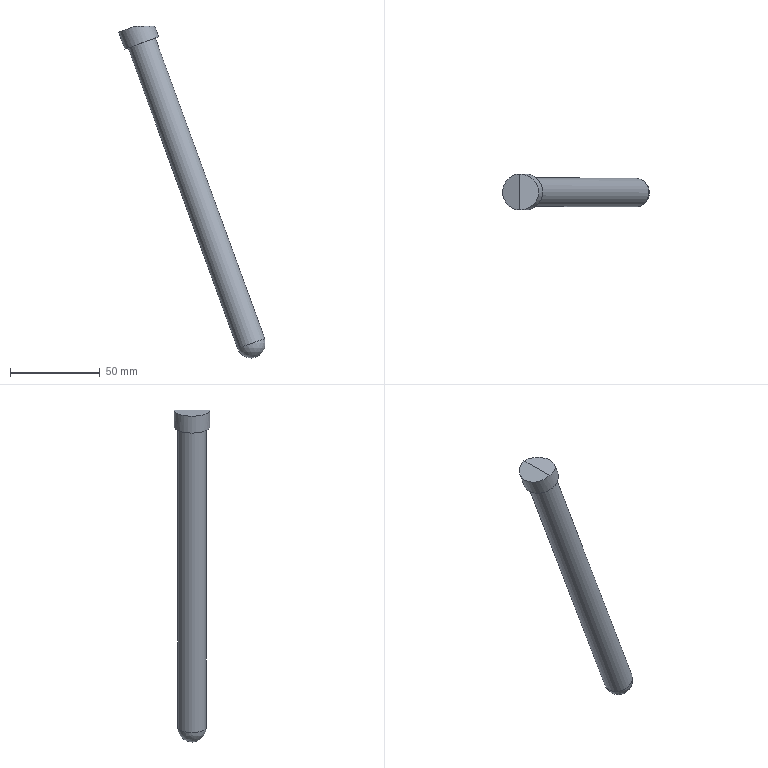Part | STEP file | lll_id310_x_t | 1 solid | 6 faces | box 81.68 x 20 x 184.615 mm | volume 39750 mm3 | plane 3 | cylinder 2 | sphere 1 | commonest cylinder face diameters 16 x1 20 x1
STEP:
#1=CARTESIAN_POINT('',(79.359,35.,81.839));
#2=VERTEX_POINT('',#1);
#3=CARTESIAN_POINT('',(71.841,35.,79.103));
#4=DIRECTION('',(0.342,0.,-0.9397));
#5=DIRECTION('',(0.9397,0.,0.342));
#6=AXIS2_PLACEMENT_3D('',#3,#4,#5);
#7=CIRCLE('',#6,8.);
#8=EDGE_CURVE('',#2,#2,#7,.T.);
#9=ORIENTED_EDGE('',*,*,#8,.T.);
#10=EDGE_LOOP('',(#9));
#11=FACE_BOUND('',#10,.T.);
#12=CARTESIAN_POINT('',(125.186,35.,-90.851));
#13=VERTEX_POINT('',#12);
#14=CARTESIAN_POINT('',(132.704,35.,-88.115));
#15=DIRECTION('',(0.342,0.,-0.9397));
#16=DIRECTION('',(-0.9397,0.,-0.342));
#17=AXIS2_PLACEMENT_3D('',#14,#15,#16);
#18=CIRCLE('',#17,8.);
#19=EDGE_CURVE('',#13,#13,#18,.T.);
#20=ORIENTED_EDGE('',*,*,#19,.F.);
#21=EDGE_LOOP('',(#20));
#22=FACE_BOUND('',#21,.T.);
#23=CARTESIAN_POINT('',(105.,35.,-12.));
#24=DIRECTION('',(-0.342,0.,0.9397));
#25=DIRECTION('',(-0.9397,0.,-0.342));
#26=AXIS2_PLACEMENT_3D('',#23,#24,#25);
#27=CYLINDRICAL_SURFACE('',#26,8.);
#28=ADVANCED_FACE('',(#11,#22),#27,.T.);
#29=ORIENTED_EDGE('',*,*,#19,.T.);
#30=EDGE_LOOP('',(#29));
#31=FACE_OUTER_BOUND('',#30,.T.);
#32=CARTESIAN_POINT('',(132.704,35.,-88.115));
#33=DIRECTION('',(0.,0.,1.));
#34=DIRECTION('',(-1.,0.,0.));
#35=AXIS2_PLACEMENT_3D('',#32,#33,#34);
#36=SPHERICAL_SURFACE('',#35,8.);
#37=ADVANCED_FACE('',(#31),#36,.T.);
#38=CARTESIAN_POINT('',(68.421,25.,88.5));
#39=VERTEX_POINT('',#38);
#40=CARTESIAN_POINT('',(68.421,45.,88.5));
#41=VERTEX_POINT('',#40);
#42=CARTESIAN_POINT('',(68.421,35.,88.5));
#43=DIRECTION('',(0.,1.,0.));
#44=VECTOR('',#43,1.);
#45=LINE('',#42,#44);
#46=EDGE_CURVE('',#39,#41,#45,.T.);
#47=ORIENTED_EDGE('',*,*,#46,.T.);
#48=CARTESIAN_POINT('',(68.421,35.,88.5));
#49=DIRECTION('',(-0.342,0.,0.9397));
#50=DIRECTION('',(0.9397,0.,0.342));
#51=AXIS2_PLACEMENT_3D('',#48,#49,#50);
#52=CIRCLE('',#51,10.);
#53=EDGE_CURVE('',#41,#39,#52,.T.);
#54=ORIENTED_EDGE('',*,*,#53,.T.);
#55=EDGE_LOOP('',(#47,#54));
#56=FACE_OUTER_BOUND('',#55,.T.);
#57=CARTESIAN_POINT('',(68.421,35.,88.5));
#58=DIRECTION('',(-0.342,0.,0.9397));
#59=DIRECTION('',(-0.9397,0.,-0.342));
#60=AXIS2_PLACEMENT_3D('',#57,#58,#59);
#61=PLANE('',#60);
#62=ADVANCED_FACE('',(#56),#61,.T.);
#63=ORIENTED_EDGE('',*,*,#8,.F.);
#64=EDGE_LOOP('',(#63));
#65=FACE_BOUND('',#64,.T.);
#66=CARTESIAN_POINT('',(62.444,35.,75.683));
#67=VERTEX_POINT('',#66);
#68=CARTESIAN_POINT('',(71.841,35.,79.103));
#69=DIRECTION('',(0.342,0.,-0.9397));
#70=DIRECTION('',(-0.9397,0.,-0.342));
#71=AXIS2_PLACEMENT_3D('',#68,#69,#70);
#72=CIRCLE('',#71,10.);
#73=EDGE_CURVE('',#67,#67,#72,.T.);
#74=ORIENTED_EDGE('',*,*,#73,.T.);
#75=EDGE_LOOP('',(#74));
#76=FACE_BOUND('',#75,.T.);
#77=CARTESIAN_POINT('',(71.841,35.,79.103));
#78=DIRECTION('',(0.342,0.,-0.9397));
#79=DIRECTION('',(0.9397,0.,0.342));
#80=AXIS2_PLACEMENT_3D('',#77,#78,#79);
#81=PLANE('',#80);
#82=ADVANCED_FACE('',(#65,#76),#81,.T.);
#83=CARTESIAN_POINT('',(68.421,35.,88.5));
#84=DIRECTION('',(0.,0.,-1.));
#85=DIRECTION('',(-1.,0.,0.));
#86=AXIS2_PLACEMENT_3D('',#83,#84,#85);
#87=ELLIPSE('',#86,10.642,10.);
#88=EDGE_CURVE('',#41,#39,#87,.T.);
#89=ORIENTED_EDGE('',*,*,#88,.T.);
#90=ORIENTED_EDGE('',*,*,#53,.F.);
#91=EDGE_LOOP('',(#89,#90));
#92=FACE_BOUND('',#91,.T.);
#93=ORIENTED_EDGE('',*,*,#73,.F.);
#94=EDGE_LOOP('',(#93));
#95=FACE_BOUND('',#94,.T.);
#96=CARTESIAN_POINT('',(71.841,35.,79.103));
#97=DIRECTION('',(-0.342,0.,0.9397));
#98=DIRECTION('',(-0.9397,0.,-0.342));
#99=AXIS2_PLACEMENT_3D('',#96,#97,#98);
#100=CYLINDRICAL_SURFACE('',#99,10.);
#101=ADVANCED_FACE('',(#92,#95),#100,.T.);
#102=ORIENTED_EDGE('',*,*,#46,.F.);
#103=ORIENTED_EDGE('',*,*,#88,.F.);
#104=EDGE_LOOP('',(#102,#103));
#105=FACE_OUTER_BOUND('',#104,.T.);
#106=CARTESIAN_POINT('',(64.053,35.,88.5));
#107=DIRECTION('',(0.,0.,-1.));
#108=DIRECTION('',(1.,0.,0.));
#109=AXIS2_PLACEMENT_3D('',#106,#107,#108);
#110=PLANE('',#109);
#111=ADVANCED_FACE('',(#105),#110,.F.);
#112=CLOSED_SHELL('',(#28,#37,#62,#82,#101,#111));
#113=MANIFOLD_SOLID_BREP('',#112);
#114=(LENGTH_UNIT()NAMED_UNIT(*)SI_UNIT(.MILLI.,.METRE.));
#115=UNCERTAINTY_MEASURE_WITH_UNIT(LENGTH_MEASURE(0.00002),#114,'','');
#116=(NAMED_UNIT(*)PLANE_ANGLE_UNIT()SI_UNIT($,.RADIAN.));
#117=PLANE_ANGLE_MEASURE_WITH_UNIT(PLANE_ANGLE_MEASURE(0.01745),#116);
#118=DIMENSIONAL_EXPONENTS(0.,0.,0.,0.,0.,0.,0.);
#119=(CONVERSION_BASED_UNIT('DEGREE',#117)NAMED_UNIT(#118)PLANE_ANGLE_UNIT());
#120=(NAMED_UNIT(*)SI_UNIT($,.STERADIAN.)SOLID_ANGLE_UNIT());
#121=(GEOMETRIC_REPRESENTATION_CONTEXT(3)GLOBAL_UNCERTAINTY_ASSIGNED_CONTEXT((#115))GLOBAL_UNIT_ASSIGNED_CONTEXT((#114,#119,#120))REPRESENTATION_CONTEXT('',''));
#122=ADVANCED_BREP_SHAPE_REPRESENTATION('',(#113),#121);